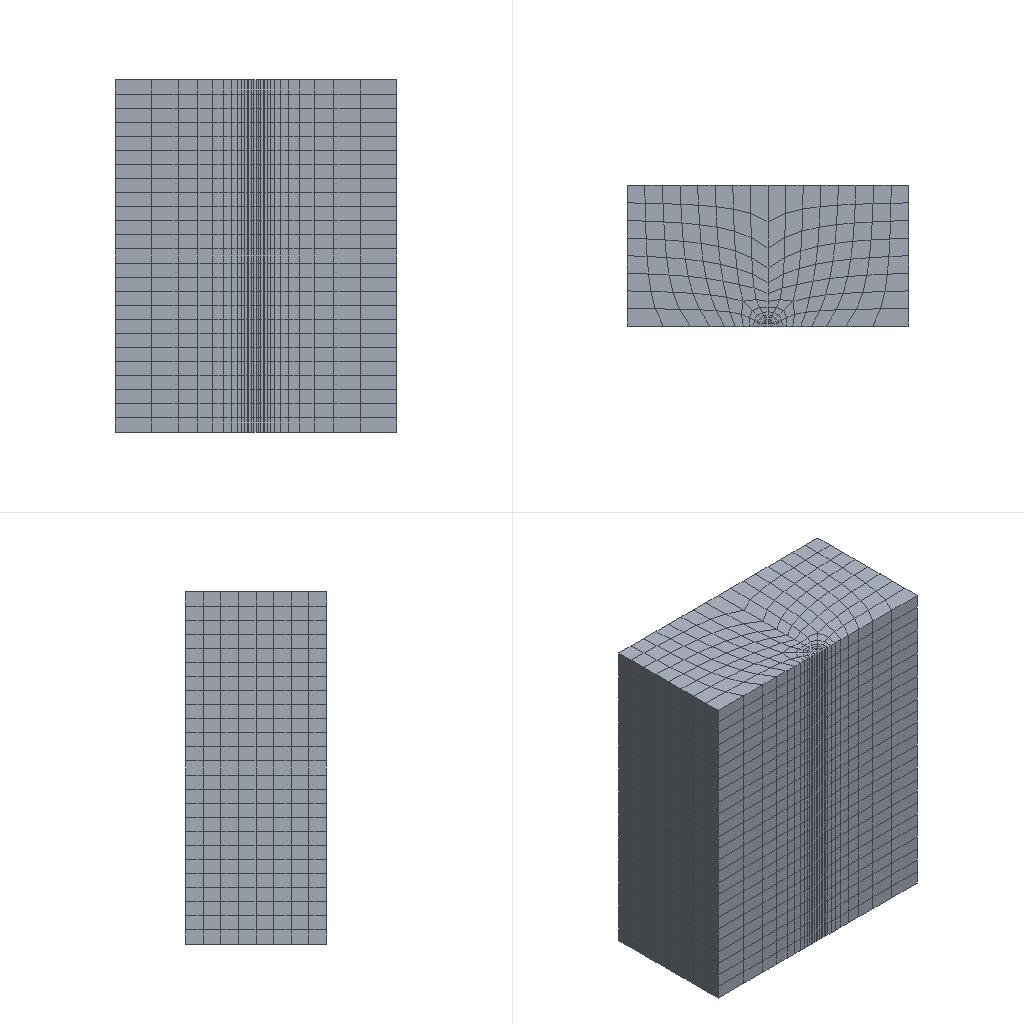Simulation study | abaqus
Set-up summary:
category,name,step,type,value,unit,region
solver,abaqus,,Abaqus/CAE 2024
units,mm-mN-s-kg (kPa) or mm-kg-s,,inferred,E=2e+07 density=
analysis,geo,,geostatic
analysis,load-v,,static,time_period=1
analysis,load-l,,static,time_period=1
mesh,nodes,,,5586
mesh,elements,,,4400
element_type,C3D8,,,4400
material,pile,,E,2e+07
material,pile,,nu,0.17
material,soil,,E,10000
material,soil,,nu,0.35
material,soil,,behaviors,plastic; mohr coulomb; mohr coulomb hardening
section,pile,,solid section,,,_PickedSet5
section,soil,,solid section,,,_PickedSet104
load,stress,initial,initial condition stress
load,Load-1,geo,bz,-18,,_PickedSet31
load,Load-2,load-v,bz,-6,,pile-1.pile
load,Load-3,load-l,shear traction,"1910 [dir=(1, 0, 0)]",,_PickedSurf27
bc,BC-1,initial,fixed,"[dofs=x,y,z n=3]",,_PickedSet32
bc,BC-2,initial,fixed,[dofs=x],,_PickedSet18
bc,BC-3,initial,fixed,[dofs=y],,_PickedSet34
contact,Int-1,initial,contact pair surface to surface,interaction=_Int-1-Prop; friction=0; behavior=hard,,soil-1.soil-l / pile-1.pile-l
contact,Int-2,initial,contact pair surface to surface,interaction=_Int-2-Prop; friction=0; behavior=hard,,soil-1.soil-b / pile-1.pile-b
Abaqus input file, long lists of numbers shortened:
*Heading
** Job name: deck Model name: Model-1
** Generated by: Abaqus/CAE 2024
*Preprint, echo=NO, model=NO, history=NO, contact=NO
**
** PARTS
**
*Part, name=pile
*Node
      1,           0.,          0.5,           2.
      2,           0.,           0.,           2.
** (502 more lines like these left out)
*Element, type=C3D8
 1, 222,  48, 219, 426,  45,   1,  47, 217
 2, 223,  49, 220, 425, 222,  48, 219, 426
** (318 more lines like these left out)
*Nset, nset=_PickedSet5, internal, generate
   1,  504,    1
*Elset, elset=_PickedSet5, internal, generate
   1,  320,    1
*Nset, nset=pile, generate
   1,  504,    1
*Elset, elset=pile, generate
   1,  320,    1
*Elset, elset=_pile-b_S2, internal, generate
 113,  120,    1
*Elset, elset=_pile-b_S3, internal, generate
  7,  10,   1
*Elset, elset=_pile-b_S4, internal
 11, 12, 15, 16
*Surface, type=ELEMENT, name=pile-b
_pile-b_S2, S2
_pile-b_S3, S3
_pile-b_S4, S4
*Elset, elset=_s1_S3, internal
 263, 264, 271, 272, 281, 282, 283, 284
*Elset, elset=_s1_S4, internal
 265, 266, 267, 268, 279, 280, 287, 288
*Surface, type=ELEMENT, name=s1
_s1_S3, S3
_s1_S4, S4
*Elset, elset=_s3_S4, internal
 197, 198, 295, 296
*Elset, elset=_s3_S3, internal
 199, 200, 205, 206, 207, 208, 297, 298, 299, 300, 303, 304
*Surface, type=ELEMENT, name=s3
_s3_S4, S4
_s3_S3, S3
*Elset, elset=_s4_S4, internal
 167, 168, 175, 176, 183, 184
*Elset, elset=_s4_S3, internal
 169, 170, 171, 172, 185, 186, 187, 188, 191, 192
*Surface, type=ELEMENT, name=s4
_s4_S4, S4
_s4_S3, S3
*Elset, elset=_s5_S4, internal
 133, 134, 145, 146, 147, 148
*Elset, elset=_s5_S3, internal
 135, 136, 141, 142, 143, 144, 149, 150
*Elset, elset=_s5_S2, internal
 157, 158
*Surface, type=ELEMENT, name=s5
_s5_S4, S4
_s5_S3, S3
_s5_S2, S2
*Elset, elset=_s6_S4, internal
 103, 104, 111, 112, 215, 216, 217, 218, 223, 224
*Elset, elset=_s6_S3, internal
 105, 106, 107, 108, 219, 220
*Surface, type=ELEMENT, name=s6
_s6_S4, S4
_s6_S3, S3
*Elset, elset=_s7_S4, internal
 69, 70, 89, 90, 95, 96
*Elset, elset=_s7_S3, internal
 71, 72, 77, 78, 79, 80, 91, 92, 93, 94
*Surface, type=ELEMENT, name=s7
_s7_S4, S4
_s7_S3, S3
*Elset, elset=_s8_S2, internal, generate
 49,  56,   1
*Elset, elset=_s8_S4, internal
 39, 40, 47, 48
*Elset, elset=_s8_S3, internal, generate
 41,  44,   1
*Surface, type=ELEMENT, name=s8
_s8_S2, S2
_s8_S4, S4
_s8_S3, S3
*Elset, elset=_s9_S4, internal
  23,  24, 305, 306
*Elset, elset=_s9_S3, internal
  25,  26,  27,  28,  31,  32, 307, 308, 309, 310
*Elset, elset=_s9_S2, internal
 317, 318
*Surface, type=ELEMENT, name=s9
_s9_S4, S4
_s9_S3, S3
_s9_S2, S2
*Elset, elset=_s10_S4, internal
   3,   4,   5,   6, 121, 122
*Elset, elset=_s10_S3, internal
   1,   2, 123, 124, 125, 126
*Elset, elset=_s10_S2, internal
  13,  14, 127, 128
*Surface, type=ELEMENT, name=s10
_s10_S4, S4
_s10_S3, S3
_s10_S2, S2
*Elset, elset=_s11_S2, internal, generate
 113,  120,    1
*Elset, elset=_s11_S3, internal, generate
  7,  10,   1
*Elset, elset=_s11_S4, internal
 11, 12, 15, 16
*Surface, type=ELEMENT, name=s11
_s11_S2, S2
_s11_S3, S3
_s11_S4, S4
*Elset, elset=_s2_S4, internal
 231, 232, 239, 240, 247, 248
*Elset, elset=_s2_S3, internal
 233, 234, 235, 236, 249, 250, 251, 252, 255, 256
*Surface, type=ELEMENT, name=s2
_s2_S4, S4
_s2_S3, S3
*Elset, elset=_pile-l_S3, internal
  11,  12,  23,  24,  39,  40,  55,  56,  81,  82,  89,  90, 103, 104, 113, 114
 121, 122, 127, 128, 151, 152, 167, 168, 183, 184, 209, 210, 221, 222, 223, 224
** (1 more lines like these left out)
*Elset, elset=_pile-l_S4, internal
   1,   2,  13,  14,  21,  22,  29,  30,  31,  32,  37,  38,  45,  46,  49,  50
  61,  62,  63,  64,  87,  88, 101, 102, 109, 110, 119, 120, 149, 150, 157, 158
** (3 more lines like these left out)
*Elset, elset=_pile-l_S2, internal
  15,  16,  47,  48,  65,  66,  67,  68,  69,  70,  71,  72,  95,  96, 111, 112
 129, 130, 131, 132, 133, 134, 135, 136, 175, 176, 193, 194, 195, 196, 197, 198
** (1 more lines like these left out)
*Surface, type=ELEMENT, name=pile-l
_pile-l_S3, S3
_pile-l_S4, S4
_pile-l_S2, S2
** Section: pile
*Solid Section, elset=_PickedSet5, material=pile
,
*End Part
**
*Part, name=soil
*Node
      1,          20.,          0.5,           5.
      2,          20.,           0.,           5.
** (5080 more lines like these left out)
*Element, type=C3D8
 1,  431,  432, 2297, 2293,   28,   29,  420,  419
 2,  432,   32,  423, 2297,   29,    1,   30,  420
** (4078 more lines like these left out)
*Nset, nset=soil, generate
    1,  5082,     1
*Elset, elset=soil, generate
    1,  4080,     1
*Nset, nset=_PickedSet104, internal, generate
    1,  5082,     1
*Elset, elset=_PickedSet104, internal, generate
    1,  4080,     1
*Elset, elset=_soil-b_S2, internal
  1,  2,  5,  6,  7,  8, 13, 14, 41, 42, 43, 44, 49, 50, 53, 54
*Surface, type=ELEMENT, name=soil-b
_soil-b_S2, S2
*Elset, elset=_soil-l_S6, internal
  903,  904,  983,  984, 1063, 1064, 1143, 1144, 1223, 1224, 1303, 1304, 1383, 1384, 1463, 1464
 1543, 1544, 1623, 1624, 1703, 1704, 1783, 1784, 1863, 1864, 1943, 1944, 2023, 2024, 2103, 2104
** (3 more lines like these left out)
*Elset, elset=_soil-l_S5, internal
  897,  902,  977,  982, 1057, 1062, 1137, 1142, 1217, 1222, 1297, 1302, 1377, 1382, 1457, 1462
 1537, 1542, 1617, 1622, 1697, 1702, 1777, 1782, 1857, 1862, 1937, 1942, 2017, 2022, 2097, 2102
** (3 more lines like these left out)
*Surface, type=ELEMENT, name=soil-l
_soil-l_S6, S6
_soil-l_S5, S5
** Section: soil
*Solid Section, elset=_PickedSet104, material=soil
,
*End Part
**
**
** ASSEMBLY
**
*Assembly, name=Assembly
**
*Instance, name=pile-1, part=pile
         20.,           0.,           5.
*End Instance
**
*Instance, name=soil-1, part=soil
*End Instance
**
*Nset, nset=_PickedSet18, internal, instance=soil-1
   10,   11,   12,   13,   15,   16,   17,   18,   21,   22,   25,   26,   94,   95,   96,   97
   98,   99,  100,  105,  106,  107,  108,  109,  110,  111,  112,  123,  124,  125,  126,  127
** (28 more lines like these left out)
*Elset, elset=_PickedSet18, internal, instance=soil-1
  118,  124,  125,  126,  127,  128,  129,  130,  198,  204,  205,  206,  207,  208,  209,  210
  278,  284,  285,  286,  287,  288,  289,  290,  358,  364,  365,  366,  367,  368,  369,  370
** (23 more lines like these left out)
*Nset, nset=_PickedSet31, internal, instance=pile-1, generate
   1,  504,    1
*Nset, nset=_PickedSet31, internal, instance=soil-1, generate
    1,  5082,     1
*Elset, elset=_PickedSet31, internal, instance=pile-1, generate
   1,  320,    1
*Elset, elset=_PickedSet31, internal, instance=soil-1, generate
    1,  4080,     1
*Nset, nset=_PickedSet32, internal, instance=soil-1
   4,   5,   6,   8,  12,  13,  14,  17,  18,  46,  47,  48,  49,  50,  51,  52
  62,  63,  64,  65,  66, 113, 114, 115, 116, 117, 118, 119, 120, 121, 122, 123
** (11 more lines like these left out)
*Elset, elset=_PickedSet32, internal, instance=soil-1
  19,  22,  23,  24,  29,  30,  37,  40,  57,  60,  65,  68,  71,  74,  75,  76
 401, 402, 403, 404, 405, 406, 407, 408, 409, 410, 411, 412, 413, 414, 415, 416
** (9 more lines like these left out)
*Nset, nset=_PickedSet33, internal, instance=pile-1, generate
   1,  504,    1
*Nset, nset=_PickedSet33, internal, instance=soil-1, generate
    1,  5082,     1
*Elset, elset=_PickedSet33, internal, instance=pile-1, generate
   1,  320,    1
*Elset, elset=_PickedSet33, internal, instance=soil-1, generate
    1,  4080,     1
*Nset, nset=_PickedSet34, internal, instance=pile-1
   2,   3,   5,   6,   8,   9,  10,  11,  12,  13,  15,  17,  18,  19,  20,  21
  23,  25,  26,  27,  28,  29,  30,  32,  34,  35,  36,  37,  39,  40,  42,  43
** (8 more lines like these left out)
*Nset, nset=_PickedSet34, internal, instance=soil-1
    2,    3,    5,    6,    7,    8,    9,   10,   11,   12,   13,   14,   15,   16,   17,   18
   20,   21,   22,   23,   24,   25,   26,   36,   37,   38,   39,   40,   41,   42,   43,   44
** (67 more lines like these left out)
*Elset, elset=_PickedSet34, internal, instance=pile-1
   3,   5,   8,  10,  13,  15,  17,  19,  26,  28,  29,  31,  33,  34,  37,  39
  41,  42,  51,  52,  56,  57,  59,  63,  65,  72,  73,  74,  77,  78,  84,  86
** (6 more lines like these left out)
*Elset, elset=_PickedSet34, internal, instance=soil-1
    6,    8,   10,   12,   13,   15,   24,   26,   28,   30,   32,   34,   35,   36,   37,   41
   42,   45,   46,   54,   56,   63,   64,   65,   69,   70,   71,   76,   78,   80,   81,   82
** (60 more lines like these left out)
*Elset, elset=__PickedSurf27_S3, internal, instance=pile-1
 263, 264, 271, 272, 281, 282, 283, 284
*Elset, elset=__PickedSurf27_S4, internal, instance=pile-1
 265, 266, 267, 268, 279, 280, 287, 288
*Surface, type=ELEMENT, name=_PickedSurf27, internal
__PickedSurf27_S3, S3
__PickedSurf27_S4, S4
*End Assembly
**
** MATERIALS
**
*Material, name=pile
*Elastic
 2e+07, 0.17
*Material, name=soil
*Elastic
10000., 0.35
*Mohr Coulomb
30.,0.
*Mohr Coulomb Hardening
10.,0.
**
** INTERACTION PROPERTIES
**
*Surface Interaction, name=_Int-1-Prop
1.,
*Friction
0.,
*Surface Behavior, pressure-overclosure=HARD
*Surface Interaction, name=_Int-2-Prop
1.,
*Friction
0.,
*Surface Behavior, pressure-overclosure=HARD
*Surface Interaction, name=free
1.,
*Friction
0.,
*Surface Behavior, pressure-overclosure=HARD
*Surface Interaction, name=ture
1.,
*Friction, elastic slip=1e-05
 0.4,
*Surface Behavior, pressure-overclosure=HARD
**
** BOUNDARY CONDITIONS
**
** Name: BC-1 Type: Displacement/Rotation
*Boundary
_PickedSet32, 1, 1
_PickedSet32, 2, 2
_PickedSet32, 3, 3
** Name: BC-2 Type: Displacement/Rotation
*Boundary
_PickedSet18, 1, 1
** Name: BC-3 Type: Displacement/Rotation
*Boundary
_PickedSet34, 2, 2
**
** PREDEFINED FIELDS
**
** Name: stress   Type: Geostatic stress
*Initial Conditions, type=STRESS, GEOSTATIC
_PickedSet33, 0., 25., -450., 0., 1., 1.
**
** INTERACTIONS
**
** Interaction: Int-1
*Contact Pair, interaction=_Int-1-Prop, small sliding, type=SURFACE TO SURFACE
soil-1.soil-l, pile-1.pile-l
** Interaction: Int-2
*Contact Pair, interaction=_Int-2-Prop, small sliding, type=SURFACE TO SURFACE
soil-1.soil-b, pile-1.pile-b
** ----------------------------------------------------------------
**
** STEP: geo
**
*Step, name=geo, nlgeom=NO, unsymm=YES
*Geostatic
**
** LOADS
**
** Name: Load-1   Type: Body force
*Dload
_PickedSet31, BZ, -18.
**
** OUTPUT REQUESTS
**
*Restart, write, frequency=0
**
** FIELD OUTPUT: F-Output-1
**
*Output, field, variable=PRESELECT
**
** HISTORY OUTPUT: H-Output-1
**
*Output, history, variable=PRESELECT
*End Step
** ----------------------------------------------------------------
**
** STEP: load-v
**
*Step, name=load-v, nlgeom=NO, unsymm=YES
*Static
0.1, 1., 1e-05, 0.5
**
** LOADS
**
** Name: Load-2   Type: Body force
*Dload
pile-1.pile, BZ, -6.
**
** INTERACTIONS
**
** Interaction: Int-1
*Change Friction, interaction=_Int-1-Prop
*Friction, elastic slip=1e-05
 0.4,
** Interaction: Int-2
*Change Friction, interaction=_Int-2-Prop
*Friction, elastic slip=1e-05
 0.4,
**
** OUTPUT REQUESTS
**
*Restart, write, frequency=0
**
** FIELD OUTPUT: F-Output-1
**
*Output, field, variable=PRESELECT
**
** HISTORY OUTPUT: H-Output-1
**
*Output, history, variable=PRESELECT
*End Step
** ----------------------------------------------------------------
**
** STEP: load-l
**
*Step, name=load-l, nlgeom=NO, unsymm=YES
*Static
0.1, 1., 1e-05, 0.5
**
** LOADS
**
** Name: Load-3   Type: Surface traction
*Dsload, constant resultant=YES
_PickedSurf27, TRSHR, 1910., 1., 0., 0.
**
** OUTPUT REQUESTS
**
*Restart, write, frequency=0
**
** FIELD OUTPUT: F-Output-1
**
*Output, field, variable=PRESELECT
**
** HISTORY OUTPUT: H-Output-1
**
*Output, history, variable=PRESELECT
*section print,name=s1,surface=pile-1.s1,axes=local,frequency=1,update=yes
,20,0,25
,30,0,25,,20,10,25
sof,som
*section print,name=s2,surface=pile-1.s2,axes=local,frequency=1,update=yes
,20,0,23
,30,0,23,,20,10,23
sof,som
*section print,name=s3,surface=pile-1.s3,axes=local,frequency=1,update=yes
,20,0,21
,30,0,21,,20,10,21
sof,som
*section print,name=s4,surface=pile-1.s4,axes=local,frequency=1,update=yes
,20,0,19
,30,0,19,,20,10,19
sof,som
*section print,name=s5,surface=pile-1.s5,axes=local,frequency=1,update=yes
,20,0,17
,30,0,17,,20,10,17
sof,som
*section print,name=s6,surface=pile-1.s6,axes=local,frequency=1,update=yes
,20,0,15
,30,0,15,,20,10,15
sof,som
*section print,name=s7,surface=pile-1.s7,axes=local,frequency=1,update=yes
,20,0,13
,30,0,13,,20,10,13
sof,som
*section print,name=s8,surface=pile-1.s8,axes=local,frequency=1,update=yes
,20,0,11
,30,0,11,,20,10,11
sof,som
*section print,name=s9,surface=pile-1.s9,axes=local,frequency=1,update=yes
,20,0,9
,30,0,9,,20,10,9
sof,som
*section print,name=s10,surface=pile-1.s10,axes=local,frequency=1,update=yes
,20,0,7
,30,0,7,,20,10,7
sof,som
*section print,name=s11,surface=pile-1.s11,axes=local,frequency=1,update=yes
,20,0,5
,30,0,5,,20,10,5
sof,som
*End Step
Results summary:
result,odb.job_status,,,JOB_STATUS_COMPLETED_SUCCESSFULLY,"consistent, unstated (Abaqus has no unit system)"
result,steps[0].procedure,geo,,*GEOSTATIC,"consistent, unstated (Abaqus has no unit system)"
result,steps[0].time_period,geo,,1,"consistent, unstated (Abaqus has no unit system)"
result,steps[0].n_frames,geo,,2,"consistent, unstated (Abaqus has no unit system)"
result,steps[0].last_frame.id,geo,,1,"consistent, unstated (Abaqus has no unit system)"
result,steps[0].last_frame.value,geo,,1,"consistent, unstated (Abaqus has no unit system)"
result,steps[0].last_frame.description,geo,,Increment      1: Step Time =    1.000,"consistent, unstated (Abaqus has no unit system)"
result,steps[0].completed,geo,,True,"consistent, unstated (Abaqus has no unit system)"
result,steps[0].max_U_magnitude,geo,,0.0002343,"consistent, unstated (Abaqus has no unit system)"
result,steps[0].max_S_mises,geo,,12.641,"consistent, unstated (Abaqus has no unit system)"
result,steps[0].RF_sum[1],geo,,-0.0118,"consistent, unstated (Abaqus has no unit system)"
result,steps[0].RF_sum[2],geo,,-0.01994,"consistent, unstated (Abaqus has no unit system)"
result,steps[0].RF_sum[3],geo,,90000,"consistent, unstated (Abaqus has no unit system)"
result,steps[1].procedure,load-v,,*STATIC,"consistent, unstated (Abaqus has no unit system)"
result,steps[1].time_period,load-v,,1,"consistent, unstated (Abaqus has no unit system)"
result,steps[1].n_frames,load-v,,9,"consistent, unstated (Abaqus has no unit system)"
result,steps[1].last_frame.id,load-v,,8,"consistent, unstated (Abaqus has no unit system)"
result,steps[1].last_frame.value,load-v,,1,"consistent, unstated (Abaqus has no unit system)"
result,steps[1].last_frame.description,load-v,,Increment      8: Step Time =    1.000,"consistent, unstated (Abaqus has no unit system)"
result,steps[1].completed,load-v,,True,"consistent, unstated (Abaqus has no unit system)"
result,steps[1].max_U_magnitude,load-v,,0.0006145,"consistent, unstated (Abaqus has no unit system)"
result,steps[1].max_S_mises,load-v,,21.946,"consistent, unstated (Abaqus has no unit system)"
result,steps[1].RF_sum[1],load-v,,0.002369,"consistent, unstated (Abaqus has no unit system)"
result,steps[1].RF_sum[2],load-v,,-0.02021,"consistent, unstated (Abaqus has no unit system)"
result,steps[1].RF_sum[3],load-v,,90045.9,"consistent, unstated (Abaqus has no unit system)"
result,steps[2].procedure,load-l,,*STATIC,"consistent, unstated (Abaqus has no unit system)"
result,steps[2].time_period,load-l,,1,"consistent, unstated (Abaqus has no unit system)"
result,steps[2].n_frames,load-l,,10,"consistent, unstated (Abaqus has no unit system)"
result,steps[2].last_frame.id,load-l,,9,"consistent, unstated (Abaqus has no unit system)"
result,steps[2].last_frame.value,load-l,,1,"consistent, unstated (Abaqus has no unit system)"
result,steps[2].last_frame.description,load-l,,Increment      9: Step Time =    1.000,"consistent, unstated (Abaqus has no unit system)"
result,steps[2].completed,load-l,,True,"consistent, unstated (Abaqus has no unit system)"
result,steps[2].max_U_magnitude,load-l,,0.1023,"consistent, unstated (Abaqus has no unit system)"
result,steps[2].max_S_mises,load-l,,24447,"consistent, unstated (Abaqus has no unit system)"
result,steps[2].RF_sum[1],load-l,,-730.927,"consistent, unstated (Abaqus has no unit system)"
result,steps[2].RF_sum[2],load-l,,0.006844,"consistent, unstated (Abaqus has no unit system)"
result,steps[2].RF_sum[3],load-l,,90045.9,"consistent, unstated (Abaqus has no unit system)"